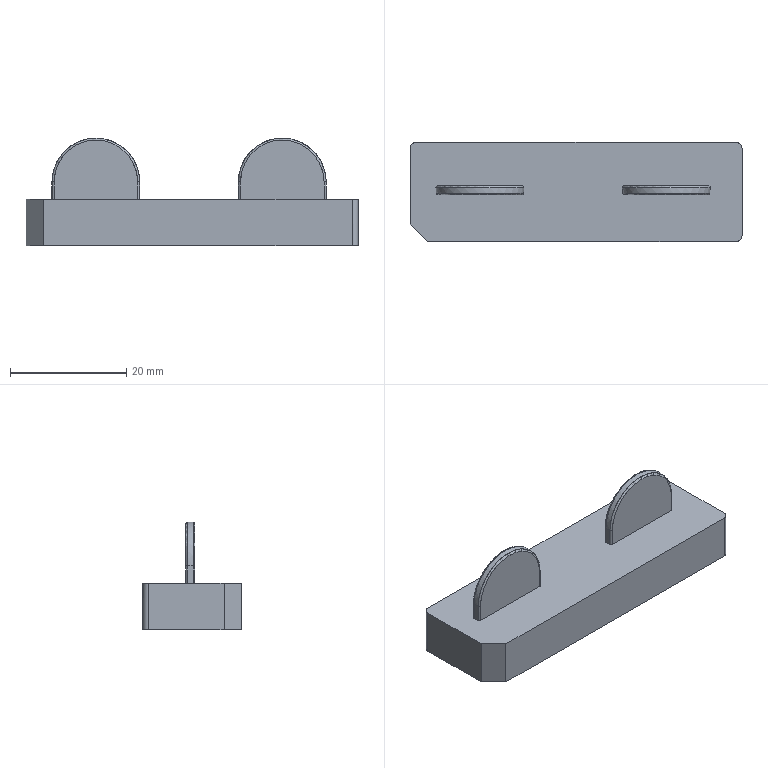NC program | PowerMill | posted by the shop | part box 57 x 17 x 18.538 mm
Lines 5023 to 6543 of 218548:
( TOOL ID   D4C_1_1 )
( TOOL DIA. 4. TIP RAD 0 LENGTH 65.72 )
( Z = -10.67 )
T2 M6
T3
G91 G28 Z0
G0 G90 G54
M08
S18000 M3
X0 Y0 M8
G43 Z9.797 H2
X-20.524 Y-1.597
Z.79
G1 Z-.41 F3600
X-20.502 Y-1.601 F6000
G3 X-20.271 Y-1.444 I.037 J.194
G1 X-20.041 Y-.244
X-20.178 Y.244
X-20.238 Y.732
X-20.172 Y1.22
X-19.971 Y1.708
X-19.766 Y2.027
X-19.624 Y2.196
X-19.278 Y2.487
X-18.904 Y2.684
X-18.302 Y2.887
X-17.814 Y2.962
X-17.326 Y3.001
X-16.35 Y3.018
X-15.374 Y2.982
X-14.886 Y2.924
X-14.398 Y2.808
X-13.91 Y2.598
X-13.421 Y2.241
X-13.026 Y1.708
X-12.829 Y1.22
X-12.765 Y.732
X-12.821 Y.244
X-13.094 Y-.732
X-13.31 Y-1.22
X-13.421 Y-1.396
X-13.706 Y-1.708
X-13.91 Y-1.865
X-14.398 Y-2.158
X-14.496 Y-2.196
X-14.886 Y-2.298
X-15.374 Y-2.385
X-16.35 Y-2.439
X-17.326 Y-2.416
X-17.814 Y-2.352
X-18.506 Y-2.196
X-18.79 Y-2.065
X-19.278 Y-1.718
X-19.693 Y-1.22
X-19.903 Y-.732
X-20.041 Y-.244
X-21.294 Y-1.636 Z-.608
X-21.273 Y-1.641
G3 X-21.032 Y-1.5 I.05 J.192
G1 X-20.741 Y-.392
X-20.875 Y.244
X-20.933 Y.732
X-20.868 Y1.22
X-20.674 Y1.708
X-20.331 Y2.196
X-20.254 Y2.274
X-19.766 Y2.62
X-19.278 Y2.838
X-18.79 Y2.963
X-18.302 Y3.016
X-14.886 Y3.03
X-14.398 Y2.988
X-13.91 Y2.89
X-13.421 Y2.723
X-12.933 Y2.431
X-12.668 Y2.196
X-12.445 Y1.914
X-12.327 Y1.708
X-12.132 Y1.22
X-12.067 Y.732
X-12.123 Y.244
X-12.33 Y-.732
X-12.538 Y-1.22
X-12.936 Y-1.708
X-13.421 Y-2.075
X-13.683 Y-2.196
X-13.91 Y-2.286
X-14.398 Y-2.401
X-14.886 Y-2.463
X-15.374 Y-2.483
X-17.326 Y-2.49
X-18.302 Y-2.442
X-18.79 Y-2.371
X-19.317 Y-2.196
X-19.766 Y-1.959
X-20.064 Y-1.708
X-20.254 Y-1.511
X-20.465 Y-1.22
X-20.67 Y-.732
X-20.741 Y-.392
X-21.833 Y-1.658 Z-.805
X-21.812 Y-1.664
G3 X-21.565 Y-1.531 I.057 J.19
G1 X-21.252 Y-.481
X-21.378 Y.244
X-21.434 Y.732
X-21.37 Y1.22
X-21.23 Y1.628
X-20.856 Y2.196
X-20.742 Y2.305
X-20.254 Y2.662
X-19.766 Y2.866
X-19.278 Y2.982
X-18.79 Y3.032
X-14.398
X-13.91 Y3.008
X-13.421 Y2.925
X-12.785 Y2.684
X-12.445 Y2.456
X-12.146 Y2.196
X-11.957 Y1.962
X-11.804 Y1.708
X-11.631 Y1.22
X-11.566 Y.732
X-11.622 Y.244
X-11.792 Y-.732
X-11.957 Y-1.144
X-12.359 Y-1.708
X-12.445 Y-1.79
X-13.073 Y-2.196
X-13.421 Y-2.331
X-13.91 Y-2.433
X-14.398 Y-2.48
X-16.287 Y-2.486
X-17.326 Y-2.49
X-17.342 Y-2.489
X-17.347
X-18.302 Y-2.492
X-18.79 Y-2.469
X-19.278 Y-2.397
X-19.766 Y-2.268
X-20.254 Y-2.018
X-20.64 Y-1.708
X-21.003 Y-1.22
X-21.208 Y-.732
X-21.252 Y-.481
X-22.247 Y-1.749 Z-1.002
X-22.226 Y-1.755
G3 X-21.983 Y-1.616 I.052 J.191
G1 X-21.698 Y-.571
X-21.718 Y-.472
X-21.863 Y.732
X-21.801 Y1.22
X-21.63 Y1.708
X-21.29 Y2.196
X-20.742 Y2.643
X-20.254 Y2.863
X-19.766 Y2.982
X-19.278 Y3.032
X-13.91
X-13.421 Y3.012
X-12.933 Y2.921
X-12.329 Y2.684
X-11.957 Y2.429
X-11.709 Y2.196
X-11.469 Y1.886
X-11.368 Y1.708
X-11.199 Y1.22
X-11.134 Y.732
X-11.333 Y-.732
X-11.538 Y-1.22
X-11.889 Y-1.708
X-12.445 Y-2.116
X-12.596 Y-2.196
X-12.933 Y-2.328
X-13.421 Y-2.444
X-13.91 Y-2.488
X-14.398 Y-2.492
X-18.79
X-19.278 Y-2.474
X-19.766 Y-2.403
X-20.254 Y-2.264
X-20.742 Y-2.006
X-21.111 Y-1.708
X-21.23 Y-1.571
X-21.462 Y-1.22
X-21.666 Y-.732
X-21.698 Y-.571
X-22.65 Y-1.714 Z-1.199
X-22.629 Y-1.721
G3 X-22.379 Y-1.594 I.062 J.188
G1 X-22.059 Y-.624
X-22.187 Y.244
X-22.242 Y.732
X-22.206 Y1.087
X-22.008 Y1.708
X-21.718 Y2.141
X-21.23 Y2.575
X-21.051 Y2.684
X-20.742 Y2.823
X-20.254 Y2.969
X-19.766 Y3.031
X-19.291
X-19.284 Y3.032
X-19.278
X-14.062
X-13.421
X-12.933 Y3.004
X-12.445 Y2.895
X-11.951 Y2.684
X-11.469 Y2.331
X-11.33 Y2.196
X-10.989 Y1.708
X-10.821 Y1.22
X-10.757 Y.732
X-10.955 Y-.732
X-11.16 Y-1.22
X-11.469 Y-1.662
X-11.957 Y-2.058
X-12.195 Y-2.196
X-12.445 Y-2.3
X-12.933 Y-2.436
X-13.421 Y-2.487
X-13.91 Y-2.492
X-19.278
X-19.766 Y-2.472
X-20.254 Y-2.391
X-20.742 Y-2.226
X-21.23 Y-1.933
X-21.49 Y-1.708
X-21.718 Y-1.424
X-21.839 Y-1.22
X-22.043 Y-.732
X-22.059 Y-.624
X-22.999 Y-1.713 Z-1.397
X-22.978 Y-1.72
G3 X-22.726 Y-1.599 I.066 J.187
G1 X-22.396 Y-.665
X-22.57 Y.732
X-22.505 Y1.22
X-22.328 Y1.708
X-22.206 Y1.919
X-21.987 Y2.196
X-21.718 Y2.459
X-21.382 Y2.684
X-20.742 Y2.94
X-20.254 Y3.027
X-19.766 Y3.032
X-12.933
X-12.445 Y2.983
X-11.957 Y2.847
X-11.469 Y2.597
X-11.012 Y2.196
X-10.672 Y1.708
X-10.497 Y1.22
X-10.431 Y.732
X-10.612 Y-.732
X-10.818 Y-1.22
X-10.981 Y-1.48
X-11.169 Y-1.708
X-11.469 Y-1.964
X-11.832 Y-2.196
X-12.445 Y-2.412
X-12.933 Y-2.479
X-13.421 Y-2.492
X-19.766
X-20.254 Y-2.463
X-20.742 Y-2.359
X-21.166 Y-2.196
X-21.718 Y-1.816
X-21.831 Y-1.708
X-22.183 Y-1.22
X-22.387 Y-.732
X-22.396 Y-.665
X-23. Y-2.199 Z-1.594
X-22.978 Y-2.201
G3 X-22.765 Y-2.019 I.015 J.197
G1 X-22.669 Y-.776
X-22.687 Y-.732
X-22.86 Y.732
X-22.8 Y1.22
X-22.633 Y1.708
X-22.206 Y2.294
X-21.718 Y2.67
X-21.23 Y2.891
X-20.742 Y3.009
X-20.254 Y3.032
X-19.766
X-12.933
X-12.904 Y3.029
X-12.445
X-11.957 Y2.943
X-11.469 Y2.766
X-10.981 Y2.468
X-10.704 Y2.196
X-10.493 Y1.926
X-10.367 Y1.708
X-10.2 Y1.22
X-10.141 Y.732
X-10.313 Y-.732
X-10.493 Y-1.183
X-10.859 Y-1.708
X-10.981 Y-1.823
X-11.523 Y-2.196
X-11.957 Y-2.364
X-12.445 Y-2.465
X-12.933 Y-2.492
X-13.42
X-13.421
X-19.766
X-19.788 Y-2.491
X-19.794
X-20.254
X-20.742 Y-2.44
X-21.23 Y-2.3
X-21.476 Y-2.196
X-21.718 Y-2.051
X-22.141 Y-1.708
X-22.488 Y-1.22
X-22.669 Y-.776
X-23.198 Y-2.283 Z-1.791
X-23.176 Y-2.284
G3 X-22.966 Y-2.098 I.012 J.198
G1 X-22.892 Y-.872
X-22.951 Y-.732
X-23.03 Y-.244
X-23.124 Y.732
X-23.059 Y1.22
X-22.89 Y1.708
X-22.694 Y2.024
X-22.556 Y2.196
X-22.206 Y2.525
X-21.718 Y2.81
X-21.23 Y2.968
X-20.742 Y3.032
X-12.445
X-11.957 Y3.007
X-11.469 Y2.884
X-11.042 Y2.684
X-10.493 Y2.251
X-10.11 Y1.708
X-10.005 Y1.454
X-9.941 Y1.22
X-9.876 Y.732
X-9.916 Y.244
X-10.049 Y-.732
X-10.243 Y-1.22
X-10.493 Y-1.598
X-10.591 Y-1.708
X-10.981 Y-2.04
X-11.239 Y-2.196
X-11.469 Y-2.295
X-11.957 Y-2.441
X-12.445 Y-2.491
X-12.915
X-12.933 Y-2.492
X-13.417
X-13.419
X-13.421
X-19.55
X-20.254
X-20.742 Y-2.477
X-21.23 Y-2.4
X-21.718 Y-2.216
X-22.206 Y-1.892
X-22.409 Y-1.708
X-22.694 Y-1.334
X-22.892 Y-.872
X-23.45 Y-2.269 Z-1.989
X-23.428 Y-2.271
G3 X-23.214 Y-2.09 I.017 J.197
G1 X-23.117 Y-.961
X-23.208 Y-.732
X-23.369 Y.732
X-23.312 Y1.22
X-23.183 Y1.625
X-22.814 Y2.196
X-22.694 Y2.327
X-22.215 Y2.684
X-21.718 Y2.907
X-21.23 Y3.017
X-20.742 Y3.032
X-20.063
X-12.445
X-12.434 Y3.031
X-12.429
X-11.957
X-11.469 Y2.957
X-10.981 Y2.79
X-10.493 Y2.493
X-10.186 Y2.196
X-10.005 Y1.962
X-9.856 Y1.708
X-9.689 Y1.22
X-9.631 Y.732
X-9.792 Y-.732
X-9.986 Y-1.22
X-10.334 Y-1.708
X-10.493 Y-1.855
X-10.983 Y-2.196
X-11.469 Y-2.387
X-11.957 Y-2.473
X-12.445 Y-2.492
X-20.742
X-21.23 Y-2.452
X-21.718 Y-2.322
X-22.018 Y-2.196
X-22.206 Y-2.088
X-22.667 Y-1.708
X-23.014 Y-1.22
X-23.117 Y-.961
X-23.619 Y-2.365 Z-2.186
X-23.597 Y-2.366
G3 X-23.385 Y-2.184 I.015 J.197
G1 X-23.3 Y-1.036
X-23.425 Y-.732
X-23.496 Y-.244
X-23.585 Y.732
X-23.527 Y1.22
X-23.36 Y1.708
X-23.183 Y2.
X-23.033 Y2.196
X-22.694 Y2.518
X-22.206 Y2.811
X-21.718 Y2.972
X-21.23 Y3.032
X-11.957
X-11.469 Y3.01
X-10.981 Y2.886
X-10.558 Y2.684
X-10.005 Y2.241
X-9.641 Y1.708
X-9.473 Y1.22
X-9.415 Y.732
X-9.504 Y-.244
X-9.574 Y-.732
X-9.762 Y-1.22
X-10.005 Y-1.591
X-10.109 Y-1.708
X-10.493 Y-2.044
X-10.747 Y-2.196
X-10.981 Y-2.301
X-11.469 Y-2.445
X-11.957 Y-2.492
X-20.742
X-21.23 Y-2.481
X-21.718 Y-2.404
X-22.206 Y-2.219
X-22.694 Y-1.893
X-22.89 Y-1.708
X-23.183 Y-1.322
X-23.3 Y-1.036
X-23.871 Y-2.329 Z-2.383
X-23.849 Y-2.332
G3 X-23.628 Y-2.16 I.025 J.196
G1 X-23.495 Y-1.105
X-23.671 Y-.605
X-23.8 Y.732
X-23.742 Y1.22
X-23.671 Y1.48
X-23.575 Y1.708
X-23.249 Y2.196
X-22.694 Y2.661
X-22.206 Y2.894
X-21.718 Y3.013
X-21.23 Y3.032
X-20.999
X-11.957
X-11.912 Y3.03
X-11.907
X-11.469
X-10.981 Y2.949
X-10.493 Y2.77
X-10.005 Y2.45
X-9.751 Y2.196
X-9.517 Y1.873
X-9.426 Y1.708
X-9.258 Y1.22
X-9.2 Y.732
X-9.237 Y.244
X-9.358 Y-.732
X-9.517 Y-1.159
X-9.893 Y-1.708
X-10.005 Y-1.815
X-10.532 Y-2.196
X-10.981 Y-2.381
X-11.469 Y-2.474
X-11.957 Y-2.492
X-21.23
X-21.718 Y-2.449
X-22.206 Y-2.313
X-22.468 Y-2.196
X-22.694 Y-2.062
X-23.106 Y-1.708
X-23.454 Y-1.22
X-23.495 Y-1.105
X-24.002 Y-2.393 Z-2.581
X-23.981 Y-2.395
G3 X-23.765 Y-2.216 I.018 J.197
G1 X-23.669 Y-1.172
X-23.84 Y-.732
X-23.911 Y-.244
X-23.994 Y.732
X-23.928 Y1.22
X-23.761 Y1.708
X-23.442 Y2.196
X-23.183 Y2.455
X-22.694 Y2.777
X-22.206 Y2.957
X-21.718 Y3.031
X-21.245
X-21.23 Y3.032
X-20.999
X-13.078
X-11.469
X-10.981 Y3.
X-10.493 Y2.86
X-10.138 Y2.684
X-10.005 Y2.593
X-9.558 Y2.196
X-9.238 Y1.708
X-9.071 Y1.22
X-9.006 Y.732
X-9.089 Y-.244
X-9.159 Y-.732
X-9.349 Y-1.22
X-9.517 Y-1.493
X-9.697 Y-1.708
X-10.005 Y-1.993
X-10.326 Y-2.196
X-10.493 Y-2.274
X-10.981 Y-2.434
X-11.469 Y-2.491
X-11.925
X-11.929
X-11.957 Y-2.492
X-20.834
X-21.276 Y-2.491
X-21.718 Y-2.477
X-22.206 Y-2.39
X-22.674 Y-2.196
X-23.183 Y-1.83
X-23.303 Y-1.708
X-23.65 Y-1.22
X-23.669 Y-1.172
X-23.913 Y-2.673 Z-2.778
X-23.891 Y-2.671
G3 X-23.71 Y-2.458 I-.016 J.197
G1 X-23.809 Y-1.257
X-23.831 Y-1.22
X-24.02 Y-.732
X-24.09 Y-.244
X-24.17 Y.732
X-24.11 Y1.22
X-23.942 Y1.708
X-23.671 Y2.136
X-23.183 Y2.589
X-23.043 Y2.684
X-22.694 Y2.858
X-22.206 Y3.
X-21.718 Y3.032
X-11.469
X-10.981 Y3.024
X-10.493 Y2.921
X-10.005 Y2.713
X-9.517 Y2.346
X-9.377 Y2.196
X-9.058 Y1.708
X-8.89 Y1.22
X-8.831 Y.732
X-8.91 Y-.244
X-8.98 Y-.732
X-9.168 Y-1.22
X-9.517 Y-1.707
X-10.005 Y-2.118
X-10.145 Y-2.196
X-10.493 Y-2.35
X-10.981 Y-2.464
X-11.469 Y-2.492
X-12.714
X-20.834
X-21.23
X-21.254 Y-2.491
X-21.257
X-21.718
X-22.206 Y-2.433
X-22.694 Y-2.272
X-22.855 Y-2.196
X-23.183 Y-1.989
X-23.484 Y-1.708
X-23.671 Y-1.485
X-23.809 Y-1.257
X-23.917 Y-2.819 Z-2.975
X-23.896 Y-2.815
G3 X-23.73 Y-2.589 I-.03 J.196
G1 X-23.924 Y-1.339
X-24.009 Y-1.22
X-24.159 Y-.834
X-24.26 Y-.244
X-24.336 Y.732
X-24.28 Y1.22
X-24.159 Y1.608
X-23.798 Y2.196
X-23.671 Y2.334
X-23.224 Y2.684
X-22.694 Y2.918
X-22.206 Y3.023
X-21.718 Y3.032
X-10.981
X-10.493 Y2.973
X-10.005 Y2.808
X-9.776 Y2.684
X-9.517 Y2.499
X-9.202 Y2.196
X-8.887 Y1.708
X-8.72 Y1.22
X-8.664 Y.732
X-8.739 Y-.244
X-8.81 Y-.732
X-8.991 Y-1.22
X-9.338 Y-1.708
X-9.517 Y-1.888
X-9.965 Y-2.196
X-10.493 Y-2.406
X-10.981 Y-2.484
X-11.469 Y-2.492
X-21.718
X-22.206 Y-2.462
X-22.694 Y-2.347
X-23.183 Y-2.114
X-23.662 Y-1.708
X-23.924 Y-1.339
X-24.021 Y-2.87 Z-3.173
X-23.999 Y-2.866
G3 X-23.834 Y-2.64 I-.03 J.196
G1 X-24.025 Y-1.411
X-24.159 Y-1.222
X-24.346 Y-.732
X-24.419 Y-.244
X-24.491 Y.732
X-24.431 Y1.22
X-24.264 Y1.708
X-23.949 Y2.196
X-23.671 Y2.469
X-23.376 Y2.684
X-23.183 Y2.79
X-22.694 Y2.968
X-22.206 Y3.032
X-10.981
X-10.493 Y3.007
X-10.005 Y2.87
X-9.624 Y2.684
X-9.051 Y2.196
X-8.736 Y1.708
X-8.568 Y1.22
X-8.51 Y.732
X-8.581 Y-.244
X-8.655 Y-.732
X-8.84 Y-1.22
X-9.029 Y-1.522
X-9.187 Y-1.708
X-9.517 Y-2.015
X-9.81 Y-2.196
X-10.005 Y-2.291
X-10.493 Y-2.441
X-10.981 Y-2.492
X-21.718
X-22.206 Y-2.483
X-22.694 Y-2.4
X-23.189 Y-2.196
X-23.671 Y-1.857
X-23.813 Y-1.708
X-24.025 Y-1.411
X-24.022 Y-2.98 Z-3.37
X-24. Y-2.975
G3 X-23.852 Y-2.738 I-.044 J.193
G1 X-24.135 Y-1.502
X-24.159 Y-1.473
X-24.312 Y-1.22
X-24.495 Y-.732
X-24.565 Y-.244
X-24.64 Y.732
X-24.582 Y1.22
X-24.416 Y1.708
X-24.159 Y2.123
X-23.671 Y2.585
X-23.528 Y2.684
X-23.183 Y2.856
X-22.694 Y3.001
X-22.206 Y3.032
X-10.981
X-10.493 Y3.024
X-10.005 Y2.922
X-9.517 Y2.711
X-9.029 Y2.336
X-8.9 Y2.196
X-8.584 Y1.708
X-8.417 Y1.22
X-8.36 Y.732
X-8.433 Y-.244
X-8.503 Y-.732
X-8.689 Y-1.22
X-9.029 Y-1.701
X-9.517 Y-2.117
X-9.659 Y-2.196
X-10.005 Y-2.353
X-10.493 Y-2.465
X-10.981 Y-2.492
X-13.02
X-21.718
X-21.73
X-22.206
X-22.694 Y-2.434
X-23.183 Y-2.275
X-23.671 Y-1.988
X-23.965 Y-1.708
X-24.135 Y-1.502
X-24.231 Y-2.917 Z-3.567
X-24.209 Y-2.914
G3 X-24.043 Y-2.689 I-.029 J.196
G1 X-24.213 Y-1.557
X-24.45 Y-1.22
X-24.629 Y-.732
X-24.699 Y-.244
X-24.77 Y.732
X-24.716 Y1.22
X-24.647 Y1.471
X-24.548 Y1.708
X-24.237 Y2.196
X-24.159 Y2.283
X-23.671 Y2.683
X-23.183 Y2.908
X-22.694 Y3.021
X-22.206 Y3.032
X-10.493
X-10.005 Y2.966
X-9.517 Y2.787
X-9.33 Y2.684
X-9.029 Y2.46
X-8.763 Y2.196
X-8.452 Y1.708
X-8.284 Y1.22
X-8.23 Y.732
X-8.301 Y-.244
X-8.371 Y-.732
X-8.55 Y-1.22
X-8.893 Y-1.708
X-9.029 Y-1.851
X-9.514 Y-2.196
X-10.005 Y-2.4
X-10.493 Y-2.483
X-10.981 Y-2.492
X-22.206
X-22.694 Y-2.459
X-23.183 Y-2.339
X-23.671 Y-2.09
X-24.107 Y-1.708
X-24.213 Y-1.557
X-24.282 Y-2.959 Z-3.764
X-24.261 Y-2.955
G3 X-24.099 Y-2.726 I-.033 J.195
G1 X-24.289 Y-1.612
X-24.576 Y-1.22
X-24.758 Y-.732
X-24.831 Y-.244
X-24.9 Y.732
X-24.841 Y1.22
X-24.674 Y1.708
X-24.362 Y2.196
X-24.159 Y2.407
X-23.671 Y2.756
X-23.183 Y2.952
X-22.694 Y3.03
X-22.287
X-22.206 Y3.032
X-10.864
X-10.493
X-10.005 Y2.996
X-9.517 Y2.844
X-9.204 Y2.684
X-9.029 Y2.56
X-8.638 Y2.196
X-8.326 Y1.708
X-8.159 Y1.22
X-8.099 Y.732
X-8.169 Y-.244
X-8.242 Y-.732
X-8.425 Y-1.22
X-8.541 Y-1.42
X-8.767 Y-1.708
X-9.029 Y-1.963
X-9.389 Y-2.196
X-9.517 Y-2.263
X-10.005 Y-2.43
X-10.493 Y-2.491
X-10.943
X-10.945
X-10.981 Y-2.492
X-21.41
X-22.206
X-22.694 Y-2.478
X-23.183 Y-2.382
X-23.611 Y-2.196
X-24.159 Y-1.789
X-24.289 Y-1.612
X-24.374 Y-2.978 Z-3.962
X-24.353 Y-2.975
G3 X-24.192 Y-2.745 I-.034 J.195
G1 X-24.38 Y-1.679
X-24.647 Y-1.319
X-24.881 Y-.732
X-24.95 Y-.244
X-25.021 Y.732
X-24.967 Y1.22
X-24.8 Y1.708
X-24.488 Y2.196
X-24.159 Y2.51
X-23.92 Y2.684
X-23.671 Y2.817
X-23.183 Y2.982
X-22.694 Y3.032
X-10.493
X-10.005 Y3.015
X-9.517 Y2.891
X-9.079 Y2.684
X-8.541 Y2.229
X-8.2 Y1.708
X-8.053 Y1.307
X-7.979 Y.732
X-8.053 Y-.319
X-8.12 Y-.732
X-8.3 Y-1.22
X-8.642 Y-1.708
X-9.029 Y-2.056
X-9.263 Y-2.196
X-9.517 Y-2.32
X-10.005 Y-2.451
X-10.493 Y-2.492
X-10.98
X-10.981
X-21.41
X-22.206
X-22.304 Y-2.489
X-22.694
X-23.183 Y-2.416
X-23.671 Y-2.231
X-24.159 Y-1.911
X-24.358 Y-1.708
X-24.38 Y-1.679
X-24.152 Y-3.149 Z-4.159
X-24.131 Y-3.142
G3 X-24.014 Y-2.887 I-.068 J.186
G1 X-24.437 Y-1.74
X-24.471 Y-1.708
X-24.647 Y-1.488
X-24.81 Y-1.22
X-24.993 Y-.732
X-25.063 Y-.244
X-25.13 Y.732
X-25.072 Y1.22
X-24.904 Y1.708
X-24.647 Y2.132
X-24.159 Y2.598
X-24.033 Y2.684
X-23.671 Y2.864
X-23.183 Y3.006
X-22.694 Y3.032
X-10.493
X-10.005 Y3.027
X-9.517 Y2.933
X-9.029 Y2.721
X-8.541 Y2.344
X-8.405 Y2.196
X-8.096 Y1.708
X-7.928 Y1.22
X-7.87 Y.732
X-7.937 Y-.244
X-8.007 Y-.732
X-8.19 Y-1.22
X-8.529 Y-1.708
X-9.029 Y-2.129
X-9.147 Y-2.196
X-9.517 Y-2.365
X-10.005 Y-2.472
X-10.493 Y-2.492
X-22.694
X-23.183 Y-2.441
X-23.671 Y-2.291
X-24.159 Y-2.002
X-24.437 Y-1.74
X-24.151 Y-3.194 Z-4.356
X-24.131 Y-3.186
G3 X-24.022 Y-2.928 I-.074 J.184
G1 X-24.481 Y-1.79
X-24.574 Y-1.708
X-24.913 Y-1.22
X-25.093 Y-.732
X-25.135 Y-.542
X-25.23 Y.732
X-25.174 Y1.22
X-25.006 Y1.708
X-24.698 Y2.196
X-24.159 Y2.669
X-23.671 Y2.903
X-23.183 Y3.019
X-22.694 Y3.032
X-17.939
X-10.493
X-10.484
X-10.005
X-9.517 Y2.964
X-9.029 Y2.776
X-8.864 Y2.684
X-8.541 Y2.438
X-8.302 Y2.196
X-7.994 Y1.708
X-7.826 Y1.22
X-7.77 Y.732
X-7.837 Y-.244
X-7.907 Y-.732
X-8.053 Y-1.148
X-8.426 Y-1.708
X-8.541 Y-1.83
X-9.044 Y-2.196
X-9.517 Y-2.396
X-10.005 Y-2.483
X-10.493 Y-2.492
X-22.694
X-23.183 Y-2.458
X-23.671 Y-2.333
X-24.159 Y-2.075
X-24.481 Y-1.79
X-24.132 Y-3.244 Z-4.554
X-24.112 Y-3.235
G3 X-24.013 Y-2.973 I-.081 J.18
G1 X-24.523 Y-1.842
X-24.647 Y-1.741
X-25.015 Y-1.22
X-25.193 Y-.732
X-25.265 Y-.244
X-25.33 Y.732
X-25.276 Y1.22
X-25.135 Y1.656
X-24.801 Y2.196
X-24.647 Y2.361
X-24.238 Y2.684
X-23.671 Y2.938
X-23.183 Y3.028
X-22.694 Y3.032
X-10.005
X-9.517 Y2.987
X-9.029 Y2.824
X-8.761 Y2.684
X-8.541 Y2.524
X-8.199 Y2.196
X-8.053 Y1.996
X-7.891 Y1.708
X-7.723 Y1.22
X-7.67 Y.732
X-7.736 Y-.244
X-7.807 Y-.732
X-7.985 Y-1.22
X-8.323 Y-1.708
X-8.541 Y-1.925
X-8.941 Y-2.196
X-9.517 Y-2.422
X-10.005 Y-2.49
X-10.394
X-10.396
X-10.493 Y-2.492
X-22.33
X-22.756 Y-2.491
X-23.183 Y-2.475
X-23.671 Y-2.37
X-24.159 Y-2.139
X-24.523 Y-1.842
X-24.091 Y-3.289 Z-4.751
X-24.071 Y-3.279
G3 X-23.986 Y-3.013 I-.091 J.176
G1 X-24.562 Y-1.896
X-24.647 Y-1.834
X-24.765 Y-1.708
X-25.102 Y-1.22
X-25.28 Y-.732
X-25.351 Y-.244
X-25.415 Y.732
X-25.359 Y1.22
X-25.192 Y1.708
X-24.885 Y2.196
X-24.647 Y2.436
X-24.327 Y2.684
X-24.159 Y2.778
X-23.671 Y2.964
X-23.183 Y3.032
X-22.7
X-22.694
X-17.404
X-10.005
X-9.517 Y3.005
X-9.029 Y2.861
X-8.673 Y2.684
X-8.541 Y2.592
X-8.115 Y2.196
X-7.808 Y1.708
X-7.641 Y1.22
X-7.585 Y.732
X-7.65 Y-.244
X-7.72 Y-.732
X-7.898 Y-1.22
X-8.053 Y-1.475
X-8.235 Y-1.708
X-8.541 Y-1.998
X-8.849 Y-2.196
X-9.029 Y-2.289
X-9.517 Y-2.441
X-10.005 Y-2.492
X-22.694
X-23.183 Y-2.484
X-23.671 Y-2.398
X-24.151 Y-2.196
X-24.562 Y-1.896
X-24.061 Y-3.326 Z-4.948
X-24.042 Y-3.315
G3 X-23.968 Y-3.045 I-.098 J.172
G1 X-24.595 Y-1.945
X-24.647 Y-1.911
X-24.847 Y-1.708
X-25.135 Y-1.309
X-25.365 Y-.732
X-25.435 Y-.244
X-25.5 Y.732
X-25.441 Y1.22
X-25.274 Y1.708
X-25.135 Y1.961
X-24.967 Y2.196
X-24.647 Y2.508
X-24.408 Y2.684
X-24.159 Y2.816
X-23.671 Y2.985
X-23.183 Y3.032
X-10.005
X-9.517 Y3.017
X-9.029 Y2.894
X-8.592 Y2.684
X-8.053 Y2.219
X-7.726 Y1.708
X-7.565 Y1.247
X-7.5 Y.732
X-7.565 Y-.116
X-7.635 Y-.732
X-7.817 Y-1.22
X-8.153 Y-1.708
X-8.541 Y-2.057
X-8.767 Y-2.196
X-9.029 Y-2.325
X-9.517 Y-2.456
X-10.005 Y-2.492
X-10.339
X-22.694
X-22.815 Y-2.49
X-22.816
X-23.183
X-23.671 Y-2.42
X-24.159 Y-2.237
X-24.595 Y-1.945
X-24.035 Y-3.356 Z-5.146
X-24.016 Y-3.344
G3 X-23.952 Y-3.071 I-.105 J.168
G1 X-24.624 Y-1.992
X-24.647 Y-1.979
X-24.929 Y-1.708
X-25.135 Y-1.44
X-25.265 Y-1.22
X-25.442 Y-.732
X-25.512 Y-.244
X-25.576 Y.732
X-25.523 Y1.22
X-25.356 Y1.708
X-25.049 Y2.196
X-24.647 Y2.575
X-24.49 Y2.684
X-24.159 Y2.851
X-23.671 Y3.002
X-23.183 Y3.032
X-10.005
X-9.517 Y3.025
X-9.029 Y2.924
X-8.541 Y2.703
X-8.053 Y2.308
X-7.952 Y2.196
X-7.644 Y1.708
X-7.565 Y1.525
X-7.477 Y1.22
X-7.424 Y.732
X-7.488 Y-.244
X-7.565 Y-.756
X-7.735 Y-1.22
X-8.053 Y-1.686
X-8.541 Y-2.11
X-8.685 Y-2.196
X-9.029 Y-2.355
X-9.517 Y-2.469
X-10.005 Y-2.492
X-23.183
X-23.671 Y-2.435
X-24.159 Y-2.278
X-24.624 Y-1.992
X-24.423 Y-3.248 Z-5.343
X-24.402 Y-3.24
G3 X-24.288 Y-2.985 I-.071 J.185
G1 X-24.654 Y-2.025
X-24.998 Y-1.708
X-25.332 Y-1.22
X-25.51 Y-.732
X-25.583 Y-.244
X-25.644 Y.732
X-25.587 Y1.22
X-25.42 Y1.708
X-25.135 Y2.171
X-24.647 Y2.625
X-24.159 Y2.879
X-23.671 Y3.013
X-23.255 Y3.031
X-22.84 Y3.032
X-10.005
X-9.854 Y3.03
X-9.853
X-9.517
X-9.029 Y2.946
X-8.541 Y2.742
X-8.053 Y2.373
X-7.886 Y2.196
X-7.58 Y1.708
X-7.413 Y1.22
X-7.356 Y.732
X-7.417 Y-.244
X-7.49 Y-.732
X-7.668 Y-1.22
X-8.002 Y-1.708
X-8.613 Y-2.196
X-9.029 Y-2.38
X-9.517 Y-2.478
X-10.005 Y-2.492
X-23.183
X-23.671 Y-2.45
X-24.159 Y-2.31
X-24.647 Y-2.031
X-24.654 Y-2.025
X-24.422 Y-3.27 Z-5.54
X-24.401 Y-3.262
G3 X-24.292 Y-3.004 I-.074 J.184
G1 X-24.675 Y-2.049
X-25.06 Y-1.708
X-25.394 Y-1.22
X-25.569 Y-.732
X-25.623 Y-.461
X-25.703 Y.732
X-25.649 Y1.22
X-25.482 Y1.708
X-25.176 Y2.196
X-24.647 Y2.668
X-24.159 Y2.904
X-23.671 Y3.02
X-23.183 Y3.032
X-16.724
X-10.005
X-9.997
X-9.517
X-9.029 Y2.964
X-8.541 Y2.775
X-8.379 Y2.684
X-8.053 Y2.431
X-7.823 Y2.196
X-7.565 Y1.799
X-7.351 Y1.22
X-7.298 Y.732
X-7.359 Y-.244
X-7.431 Y-.732
X-7.565 Y-1.133
X-7.94 Y-1.708
X-8.053 Y-1.829
X-8.551 Y-2.196
X-9.029 Y-2.397
X-9.517 Y-2.484
X-10.005 Y-2.492
X-23.183
X-23.671 Y-2.46
X-24.159 Y-2.335
X-24.647 Y-2.075
X-24.675 Y-2.049
X-24.417 Y-3.292 Z-5.737
X-24.397 Y-3.283
G3 X-24.292 Y-3.024 I-.077 J.182
G1 X-24.695 Y-2.072
X-25.122 Y-1.708
X-25.456 Y-1.22
X-25.623 Y-.764
X-25.7 Y-.244
X-25.764 Y.732
X-25.71 Y1.22
X-25.623 Y1.526
X-25.544 Y1.708
X-25.239 Y2.196
X-25.135 Y2.312
X-24.683 Y2.684
X-24.159 Y2.926
X-23.671 Y3.026
X-23.183 Y3.032
X-9.517
X-9.029 Y2.98
X-8.541 Y2.805
X-8.317 Y2.684
X-8.053 Y2.486
X-7.761 Y2.196
X-7.565 Y1.914
X-7.456 Y1.708
X-7.289 Y1.22
X-7.236 Y.732
X-7.3 Y-.244
X-7.369 Y-.732
X-7.544 Y-1.22
X-7.878 Y-1.708
X-8.053 Y-1.888
X-8.488 Y-2.196
X-9.029 Y-2.414
X-9.517 Y-2.489
X-9.829
X-9.831
X-10.005 Y-2.492
X-22.926
X-23.183
X-23.671 Y-2.47
X-24.159 Y-2.359
X-24.647 Y-2.114
X-24.695 Y-2.072
X-24.361 Y-3.322 Z-5.935
X-24.341 Y-3.313
G3 X-24.248 Y-3.049 I-.085 J.179
G1 X-24.707 Y-2.087
X-25.135 Y-1.753
X-25.507 Y-1.22
X-25.684 Y-.732
X-25.753 Y-.244
X-25.814 Y.732
X-25.76 Y1.22
X-25.623 Y1.645
X-25.289 Y2.196
X-25.135 Y2.361
X-24.735 Y2.684
X-24.159 Y2.945
X-23.671 Y3.03
X-23.378
X-23.183 Y3.032
X-9.839
X-9.517
X-9.029 Y2.991
X-8.541 Y2.827
X-8.265 Y2.684
X-8.053 Y2.53
X-7.711 Y2.196
X-7.565 Y1.995
X-7.407 Y1.708
X-7.24 Y1.22
X-7.184 Y.732
X-7.246 Y-.244
X-7.316 Y-.732
X-7.493 Y-1.22
X-7.825 Y-1.708
X-8.053 Y-1.935
X-8.434 Y-2.196
X-8.541 Y-2.255
X-9.029 Y-2.425
X-9.517 Y-2.491
X-9.945
X-9.946
X-10.005 Y-2.492
X-21.82
X-23.183
X-23.671 Y-2.477
X-24.159 Y-2.377
X-24.566 Y-2.196
X-24.707 Y-2.087
X-24.363 Y-3.334 Z-6.132
X-24.343 Y-3.324
G3 X-24.254 Y-3.059 I-.088 J.177
G1 X-24.724 Y-2.11
X-25.135 Y-1.8
X-25.551 Y-1.22
X-25.73 Y-.732
X-25.802 Y-.244
X-25.861 Y.732
X-25.804 Y1.22
X-25.637 Y1.708
X-25.333 Y2.196
X-25.135 Y2.402
X-24.778 Y2.684
X-24.647 Y2.759
X-24.159 Y2.957
X-23.671 Y3.031
X-23.236
X-23.183 Y3.032
X-11.567
X-9.517
X-9.029 Y2.999
X-8.541 Y2.846
X-8.222 Y2.684
X-8.053 Y2.565
X-7.668 Y2.196
X-7.565 Y2.061
X-7.363 Y1.708
X-7.196 Y1.22
X-7.138 Y.732
X-7.199 Y-.244
X-7.27 Y-.732
X-7.449 Y-1.22
X-7.565 Y-1.419
X-7.782 Y-1.708
X-8.053 Y-1.97
X-8.39 Y-2.196
X-8.541 Y-2.275
X-9.029 Y-2.434
X-9.517 Y-2.492
X-23.183
X-23.671 Y-2.482
X-24.159 Y-2.39
X-24.61 Y-2.196
X-24.724 Y-2.11
X-24.36 Y-3.347 Z-6.329
X-24.34 Y-3.337
G3 X-24.255 Y-3.07 I-.091 J.176
G1 X-24.74 Y-2.131
X-25.135 Y-1.843
X-25.262 Y-1.708
X-25.595 Y-1.22
X-25.769 Y-.732
X-25.84 Y-.244
X-25.901 Y.732
X-25.848 Y1.22
X-25.681 Y1.708
X-25.376 Y2.196
X-25.135 Y2.442
X-24.822 Y2.684
X-24.647 Y2.782
X-24.159 Y2.969
X-23.671 Y3.032
X-9.517
X-9.029 Y3.007
X-8.541 Y2.866
X-8.053 Y2.599
X-7.625 Y2.196
X-7.319 Y1.708
X-7.152 Y1.22
X-7.099 Y.732
X-7.159 Y-.244
X-7.23 Y-.732
X-7.405 Y-1.22
X-7.565 Y-1.481
X-7.739 Y-1.708
X-8.053 Y-2.004
X-8.346 Y-2.196
X-8.541 Y-2.295
X-9.029 Y-2.444
X-9.517 Y-2.492
X-23.183
X-23.671 Y-2.486
X-24.159 Y-2.403
X-24.647 Y-2.2
X-24.74 Y-2.131
X-24.347 Y-3.359 Z-6.527
X-24.327 Y-3.348
G3 X-24.247 Y-3.08 I-.094 J.174
G1 X-24.751 Y-2.148
X-25.135 Y-1.879
X-25.3 Y-1.708
X-25.631 Y-1.22
X-25.807 Y-.732
X-25.877 Y-.244
X-25.937 Y.732
X-25.883 Y1.22
X-25.716 Y1.708
X-25.623 Y1.889
X-25.412 Y2.196
X-25.135 Y2.477
X-24.86 Y2.684
X-24.647 Y2.8
X-24.159 Y2.977
X-23.671 Y3.032
X-9.517
X-9.029 Y3.013
X-8.541 Y2.88
X-8.14 Y2.684
X-7.588 Y2.196
X-7.284 Y1.708
X-7.117 Y1.22
X-7.063 Y.732
X-7.123 Y-.244
X-7.193 Y-.732
X-7.369 Y-1.22
X-7.7 Y-1.708
X-8.053 Y-2.032
X-8.308 Y-2.196
X-8.541 Y-2.313
X-9.029 Y-2.451
X-9.517 Y-2.492
X-9.767
X-23.183
X-23.437 Y-2.489
X-23.438
X-23.671
X-24.159 Y-2.412
X-24.647 Y-2.221
X-24.751 Y-2.148
X-24.339 Y-3.368 Z-6.724
X-24.32 Y-3.357
G3 X-24.243 Y-3.088 I-.096 J.173
G1 X-24.759 Y-2.159
X-25.135 Y-1.902
X-25.326 Y-1.708
X-25.623 Y-1.285
X-25.836 Y-.732
X-25.906 Y-.244
X-25.967 Y.732
X-25.909 Y1.22
X-25.742 Y1.708
X-25.623 Y1.934
X-25.438 Y2.196
X-25.135 Y2.499
X-24.886 Y2.684
X-24.647 Y2.812
X-24.159 Y2.985
X-23.671 Y3.032
X-9.517
X-9.029 Y3.017
X-8.541 Y2.894
X-8.114 Y2.684
X-7.562 Y2.196
X-7.258 Y1.708
X-7.091 Y1.22
X-7.034 Y.732
X-7.094 Y-.244
X-7.164 Y-.732
X-7.343 Y-1.22
X-7.674 Y-1.708
X-8.053 Y-2.05
X-8.281 Y-2.196
X-8.541 Y-2.324
X-9.029 Y-2.456
X-9.517 Y-2.492
X-10.172
X-23.183
X-23.37 Y-2.49
X-23.371
X-23.671
X-24.159 Y-2.419
X-24.647 Y-2.236
X-24.759 Y-2.159
X-24.329 Y-3.376 Z-6.921
X-24.31 Y-3.365
G3 X-24.237 Y-3.094 I-.098 J.172
G1 X-24.766 Y-2.17
X-25.135 Y-1.925
X-25.352 Y-1.708
X-25.683 Y-1.22
X-25.861 Y-.732
X-25.932 Y-.244
X-25.991 Y.732
X-25.935 Y1.22
X-25.768 Y1.708
X-25.623 Y1.977
X-25.464 Y2.196
X-25.135 Y2.521
X-24.912 Y2.684
X-24.647 Y2.823
X-24.159 Y2.988
X-23.671 Y3.032
X-9.517
X-9.029 Y3.02
X-8.541 Y2.903
X-8.088 Y2.684
X-7.565 Y2.23
X-7.232 Y1.708
X-7.077 Y1.274
X-7.008 Y.732
X-7.077 Y-.384
X-7.139 Y-.732
X-7.317 Y-1.22
X-7.648 Y-1.708
X-8.053 Y-2.067
X-8.255 Y-2.196
X-8.541 Y-2.334
X-9.029 Y-2.462
X-9.517 Y-2.492
X-10.94
X-23.183
X-23.304 Y-2.49
X-23.305
X-23.671
X-24.159 Y-2.424
X-24.647 Y-2.25
X-24.766 Y-2.17
X-24.315 Y-3.384 Z-7.119
X-24.296 Y-3.372
G3 X-24.226 Y-3.101 I-.101 J.17
G1 X-24.772 Y-2.178
X-25.135 Y-1.944
X-25.373 Y-1.708
X-25.623 Y-1.37
X-25.703 Y-1.22
X-25.879 Y-.732
X-25.949 Y-.244
X-26.008 Y.732
X-25.957 Y1.22
X-25.789 Y1.708
X-25.623 Y2.014
X-25.486 Y2.196
X-25.135 Y2.54
X-24.933 Y2.684
X-24.647 Y2.834
X-24.159 Y2.991
X-23.671 Y3.032
X-9.517